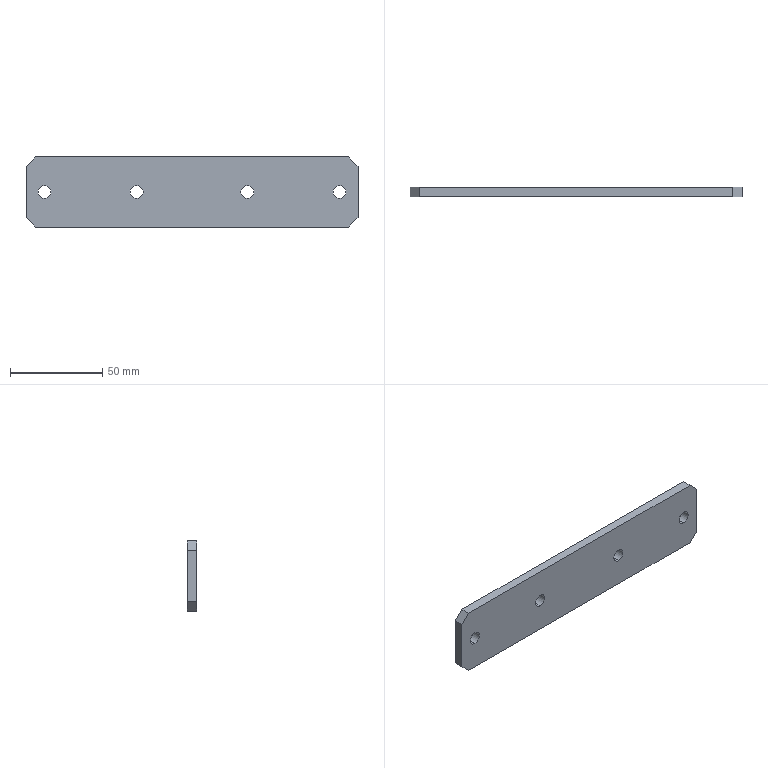Part | NX | features BREP 1 | 1 solid | 18 faces | box 180 x 5 x 38 mm | volume 33180 mm3 | plane 10 | cylinder 8 | commonest cylinder face diameters 7 x8
STEP:
#1=CARTESIAN_POINT('',(85.,5.,19.));
#2=VERTEX_POINT('',#1);
#3=CARTESIAN_POINT('',(90.,5.,14.));
#4=VERTEX_POINT('',#3);
#5=CARTESIAN_POINT('',(52.,5.,52.));
#6=DIRECTION('',(0.7071,0.,-0.7071));
#7=VECTOR('',#6,1000.);
#8=LINE('',#5,#7);
#9=EDGE_CURVE('',#2,#4,#8,.T.);
#10=ORIENTED_EDGE('',*,*,#9,.F.);
#11=CARTESIAN_POINT('',(85.,0.,19.));
#12=VERTEX_POINT('',#11);
#13=CARTESIAN_POINT('',(85.,5.,19.));
#14=DIRECTION('',(0.,1.,0.));
#15=VECTOR('',#14,1000.);
#16=LINE('',#13,#15);
#17=EDGE_CURVE('',#12,#2,#16,.T.);
#18=ORIENTED_EDGE('',*,*,#17,.F.);
#19=CARTESIAN_POINT('',(90.,0.,14.));
#20=VERTEX_POINT('',#19);
#21=CARTESIAN_POINT('',(90.,0.,14.));
#22=DIRECTION('',(-0.7071,0.,0.7071));
#23=VECTOR('',#22,1000.);
#24=LINE('',#21,#23);
#25=EDGE_CURVE('',#20,#12,#24,.T.);
#26=ORIENTED_EDGE('',*,*,#25,.F.);
#27=CARTESIAN_POINT('',(90.,5.,14.));
#28=DIRECTION('',(0.,-1.,0.));
#29=VECTOR('',#28,1000.);
#30=LINE('',#27,#29);
#31=EDGE_CURVE('',#4,#20,#30,.T.);
#32=ORIENTED_EDGE('',*,*,#31,.F.);
#33=EDGE_LOOP('',(#10,#18,#26,#32));
#34=FACE_BOUND('',#33,.T.);
#35=CARTESIAN_POINT('',(90.,5.,14.));
#36=DIRECTION('',(-0.7071,0.,-0.7071));
#37=DIRECTION('',(0.,-1.,0.));
#38=AXIS2_PLACEMENT_3D('',#35,#36,#37);
#39=PLANE('',#38);
#40=ADVANCED_FACE('',(#34),#39,.F.);
#41=CARTESIAN_POINT('',(90.,5.,-14.));
#42=VERTEX_POINT('',#41);
#43=CARTESIAN_POINT('',(85.,5.,-19.));
#44=VERTEX_POINT('',#43);
#45=CARTESIAN_POINT('',(52.,5.,-52.));
#46=DIRECTION('',(-0.7071,0.,-0.7071));
#47=VECTOR('',#46,1000.);
#48=LINE('',#45,#47);
#49=EDGE_CURVE('',#42,#44,#48,.T.);
#50=ORIENTED_EDGE('',*,*,#49,.F.);
#51=CARTESIAN_POINT('',(90.,0.,-14.));
#52=VERTEX_POINT('',#51);
#53=CARTESIAN_POINT('',(90.,5.,-14.));
#54=DIRECTION('',(0.,1.,0.));
#55=VECTOR('',#54,1000.);
#56=LINE('',#53,#55);
#57=EDGE_CURVE('',#52,#42,#56,.T.);
#58=ORIENTED_EDGE('',*,*,#57,.F.);
#59=CARTESIAN_POINT('',(85.,0.,-19.));
#60=VERTEX_POINT('',#59);
#61=CARTESIAN_POINT('',(85.,0.,-19.));
#62=DIRECTION('',(0.7071,0.,0.7071));
#63=VECTOR('',#62,1000.);
#64=LINE('',#61,#63);
#65=EDGE_CURVE('',#60,#52,#64,.T.);
#66=ORIENTED_EDGE('',*,*,#65,.F.);
#67=CARTESIAN_POINT('',(85.,5.,-19.));
#68=DIRECTION('',(0.,-1.,0.));
#69=VECTOR('',#68,1000.);
#70=LINE('',#67,#69);
#71=EDGE_CURVE('',#44,#60,#70,.T.);
#72=ORIENTED_EDGE('',*,*,#71,.F.);
#73=EDGE_LOOP('',(#50,#58,#66,#72));
#74=FACE_BOUND('',#73,.T.);
#75=CARTESIAN_POINT('',(85.,5.,-19.));
#76=DIRECTION('',(-0.7071,0.,0.7071));
#77=DIRECTION('',(0.,-1.,0.));
#78=AXIS2_PLACEMENT_3D('',#75,#76,#77);
#79=PLANE('',#78);
#80=ADVANCED_FACE('',(#74),#79,.F.);
#81=CARTESIAN_POINT('',(-90.,5.,14.));
#82=VERTEX_POINT('',#81);
#83=CARTESIAN_POINT('',(-85.,5.,19.));
#84=VERTEX_POINT('',#83);
#85=CARTESIAN_POINT('',(-52.,5.,52.));
#86=DIRECTION('',(0.7071,0.,0.7071));
#87=VECTOR('',#86,1000.);
#88=LINE('',#85,#87);
#89=EDGE_CURVE('',#82,#84,#88,.T.);
#90=ORIENTED_EDGE('',*,*,#89,.F.);
#91=CARTESIAN_POINT('',(-90.,0.,14.));
#92=VERTEX_POINT('',#91);
#93=CARTESIAN_POINT('',(-90.,5.,14.));
#94=DIRECTION('',(0.,1.,0.));
#95=VECTOR('',#94,1000.);
#96=LINE('',#93,#95);
#97=EDGE_CURVE('',#92,#82,#96,.T.);
#98=ORIENTED_EDGE('',*,*,#97,.F.);
#99=CARTESIAN_POINT('',(-85.,0.,19.));
#100=VERTEX_POINT('',#99);
#101=CARTESIAN_POINT('',(-85.,0.,19.));
#102=DIRECTION('',(-0.7071,0.,-0.7071));
#103=VECTOR('',#102,1000.);
#104=LINE('',#101,#103);
#105=EDGE_CURVE('',#100,#92,#104,.T.);
#106=ORIENTED_EDGE('',*,*,#105,.F.);
#107=CARTESIAN_POINT('',(-85.,5.,19.));
#108=DIRECTION('',(0.,-1.,0.));
#109=VECTOR('',#108,1000.);
#110=LINE('',#107,#109);
#111=EDGE_CURVE('',#84,#100,#110,.T.);
#112=ORIENTED_EDGE('',*,*,#111,.F.);
#113=EDGE_LOOP('',(#90,#98,#106,#112));
#114=FACE_BOUND('',#113,.T.);
#115=CARTESIAN_POINT('',(-85.,5.,19.));
#116=DIRECTION('',(0.7071,0.,-0.7071));
#117=DIRECTION('',(0.,-1.,0.));
#118=AXIS2_PLACEMENT_3D('',#115,#116,#117);
#119=PLANE('',#118);
#120=ADVANCED_FACE('',(#114),#119,.F.);
#121=CARTESIAN_POINT('',(-85.,5.,-19.));
#122=VERTEX_POINT('',#121);
#123=CARTESIAN_POINT('',(-90.,5.,-14.));
#124=VERTEX_POINT('',#123);
#125=CARTESIAN_POINT('',(-52.,5.,-52.));
#126=DIRECTION('',(-0.7071,0.,0.7071));
#127=VECTOR('',#126,1000.);
#128=LINE('',#125,#127);
#129=EDGE_CURVE('',#122,#124,#128,.T.);
#130=ORIENTED_EDGE('',*,*,#129,.F.);
#131=CARTESIAN_POINT('',(-85.,0.,-19.));
#132=VERTEX_POINT('',#131);
#133=CARTESIAN_POINT('',(-85.,5.,-19.));
#134=DIRECTION('',(0.,1.,0.));
#135=VECTOR('',#134,1000.);
#136=LINE('',#133,#135);
#137=EDGE_CURVE('',#132,#122,#136,.T.);
#138=ORIENTED_EDGE('',*,*,#137,.F.);
#139=CARTESIAN_POINT('',(-90.,0.,-14.));
#140=VERTEX_POINT('',#139);
#141=CARTESIAN_POINT('',(-90.,0.,-14.));
#142=DIRECTION('',(0.7071,0.,-0.7071));
#143=VECTOR('',#142,1000.);
#144=LINE('',#141,#143);
#145=EDGE_CURVE('',#140,#132,#144,.T.);
#146=ORIENTED_EDGE('',*,*,#145,.F.);
#147=CARTESIAN_POINT('',(-90.,5.,-14.));
#148=DIRECTION('',(0.,-1.,0.));
#149=VECTOR('',#148,1000.);
#150=LINE('',#147,#149);
#151=EDGE_CURVE('',#124,#140,#150,.T.);
#152=ORIENTED_EDGE('',*,*,#151,.F.);
#153=EDGE_LOOP('',(#130,#138,#146,#152));
#154=FACE_BOUND('',#153,.T.);
#155=CARTESIAN_POINT('',(-90.,5.,-14.));
#156=DIRECTION('',(0.7071,0.,0.7071));
#157=DIRECTION('',(0.,-1.,0.));
#158=AXIS2_PLACEMENT_3D('',#155,#156,#157);
#159=PLANE('',#158);
#160=ADVANCED_FACE('',(#154),#159,.F.);
#161=CARTESIAN_POINT('',(-80.,5.,-3.5));
#162=VERTEX_POINT('',#161);
#163=CARTESIAN_POINT('',(-80.,0.,-3.5));
#164=VERTEX_POINT('',#163);
#165=CARTESIAN_POINT('',(-80.,5.,-3.5));
#166=DIRECTION('',(0.,1.,0.));
#167=VECTOR('',#166,1000.);
#168=LINE('',#165,#167);
#169=EDGE_CURVE('',#162,#164,#168,.F.);
#170=ORIENTED_EDGE('',*,*,#169,.T.);
#171=CARTESIAN_POINT('',(-80.,0.,3.5));
#172=VERTEX_POINT('',#171);
#173=CARTESIAN_POINT('',(-80.,0.,0.));
#174=DIRECTION('',(0.,1.,0.));
#175=DIRECTION('',(0.,0.,1.));
#176=AXIS2_PLACEMENT_3D('',#173,#174,#175);
#177=CIRCLE('',#176,3.5);
#178=EDGE_CURVE('',#172,#164,#177,.T.);
#179=ORIENTED_EDGE('',*,*,#178,.F.);
#180=CARTESIAN_POINT('',(-80.,5.,3.5));
#181=VERTEX_POINT('',#180);
#182=CARTESIAN_POINT('',(-80.,5.,3.5));
#183=DIRECTION('',(0.,1.,0.));
#184=VECTOR('',#183,1000.);
#185=LINE('',#182,#184);
#186=EDGE_CURVE('',#181,#172,#185,.F.);
#187=ORIENTED_EDGE('',*,*,#186,.F.);
#188=CARTESIAN_POINT('',(-80.,5.,0.));
#189=DIRECTION('',(0.,1.,0.));
#190=DIRECTION('',(0.,0.,1.));
#191=AXIS2_PLACEMENT_3D('',#188,#189,#190);
#192=CIRCLE('',#191,3.5);
#193=EDGE_CURVE('',#181,#162,#192,.T.);
#194=ORIENTED_EDGE('',*,*,#193,.T.);
#195=EDGE_LOOP('',(#170,#179,#187,#194));
#196=FACE_BOUND('',#195,.T.);
#197=CARTESIAN_POINT('',(-80.,5.,0.));
#198=DIRECTION('',(0.,1.,0.));
#199=DIRECTION('',(0.,0.,1.));
#200=AXIS2_PLACEMENT_3D('',#197,#198,#199);
#201=CYLINDRICAL_SURFACE('',#200,3.5);
#202=ADVANCED_FACE('',(#196),#201,.F.);
#203=CARTESIAN_POINT('',(-30.,5.,-3.5));
#204=VERTEX_POINT('',#203);
#205=CARTESIAN_POINT('',(-30.,0.,-3.5));
#206=VERTEX_POINT('',#205);
#207=CARTESIAN_POINT('',(-30.,5.,-3.5));
#208=DIRECTION('',(0.,1.,0.));
#209=VECTOR('',#208,1000.);
#210=LINE('',#207,#209);
#211=EDGE_CURVE('',#204,#206,#210,.F.);
#212=ORIENTED_EDGE('',*,*,#211,.T.);
#213=CARTESIAN_POINT('',(-30.,0.,3.5));
#214=VERTEX_POINT('',#213);
#215=CARTESIAN_POINT('',(-30.,0.,0.));
#216=DIRECTION('',(0.,1.,0.));
#217=DIRECTION('',(0.,0.,1.));
#218=AXIS2_PLACEMENT_3D('',#215,#216,#217);
#219=CIRCLE('',#218,3.5);
#220=EDGE_CURVE('',#214,#206,#219,.T.);
#221=ORIENTED_EDGE('',*,*,#220,.F.);
#222=CARTESIAN_POINT('',(-30.,5.,3.5));
#223=VERTEX_POINT('',#222);
#224=CARTESIAN_POINT('',(-30.,5.,3.5));
#225=DIRECTION('',(0.,1.,0.));
#226=VECTOR('',#225,1000.);
#227=LINE('',#224,#226);
#228=EDGE_CURVE('',#223,#214,#227,.F.);
#229=ORIENTED_EDGE('',*,*,#228,.F.);
#230=CARTESIAN_POINT('',(-30.,5.,0.));
#231=DIRECTION('',(0.,1.,0.));
#232=DIRECTION('',(0.,0.,1.));
#233=AXIS2_PLACEMENT_3D('',#230,#231,#232);
#234=CIRCLE('',#233,3.5);
#235=EDGE_CURVE('',#223,#204,#234,.T.);
#236=ORIENTED_EDGE('',*,*,#235,.T.);
#237=EDGE_LOOP('',(#212,#221,#229,#236));
#238=FACE_BOUND('',#237,.T.);
#239=CARTESIAN_POINT('',(-30.,5.,0.));
#240=DIRECTION('',(0.,1.,0.));
#241=DIRECTION('',(0.,0.,1.));
#242=AXIS2_PLACEMENT_3D('',#239,#240,#241);
#243=CYLINDRICAL_SURFACE('',#242,3.5);
#244=ADVANCED_FACE('',(#238),#243,.F.);
#245=CARTESIAN_POINT('',(30.,5.,-3.5));
#246=VERTEX_POINT('',#245);
#247=CARTESIAN_POINT('',(30.,0.,-3.5));
#248=VERTEX_POINT('',#247);
#249=CARTESIAN_POINT('',(30.,5.,-3.5));
#250=DIRECTION('',(0.,1.,0.));
#251=VECTOR('',#250,1000.);
#252=LINE('',#249,#251);
#253=EDGE_CURVE('',#246,#248,#252,.F.);
#254=ORIENTED_EDGE('',*,*,#253,.T.);
#255=CARTESIAN_POINT('',(30.,0.,3.5));
#256=VERTEX_POINT('',#255);
#257=CARTESIAN_POINT('',(30.,0.,0.));
#258=DIRECTION('',(0.,1.,0.));
#259=DIRECTION('',(0.,0.,1.));
#260=AXIS2_PLACEMENT_3D('',#257,#258,#259);
#261=CIRCLE('',#260,3.5);
#262=EDGE_CURVE('',#256,#248,#261,.T.);
#263=ORIENTED_EDGE('',*,*,#262,.F.);
#264=CARTESIAN_POINT('',(30.,5.,3.5));
#265=VERTEX_POINT('',#264);
#266=CARTESIAN_POINT('',(30.,5.,3.5));
#267=DIRECTION('',(0.,1.,0.));
#268=VECTOR('',#267,1000.);
#269=LINE('',#266,#268);
#270=EDGE_CURVE('',#265,#256,#269,.F.);
#271=ORIENTED_EDGE('',*,*,#270,.F.);
#272=CARTESIAN_POINT('',(30.,5.,0.));
#273=DIRECTION('',(0.,1.,0.));
#274=DIRECTION('',(0.,0.,1.));
#275=AXIS2_PLACEMENT_3D('',#272,#273,#274);
#276=CIRCLE('',#275,3.5);
#277=EDGE_CURVE('',#265,#246,#276,.T.);
#278=ORIENTED_EDGE('',*,*,#277,.T.);
#279=EDGE_LOOP('',(#254,#263,#271,#278));
#280=FACE_BOUND('',#279,.T.);
#281=CARTESIAN_POINT('',(30.,5.,0.));
#282=DIRECTION('',(0.,1.,0.));
#283=DIRECTION('',(0.,0.,1.));
#284=AXIS2_PLACEMENT_3D('',#281,#282,#283);
#285=CYLINDRICAL_SURFACE('',#284,3.5);
#286=ADVANCED_FACE('',(#280),#285,.F.);
#287=CARTESIAN_POINT('',(80.,5.,-3.5));
#288=VERTEX_POINT('',#287);
#289=CARTESIAN_POINT('',(80.,0.,-3.5));
#290=VERTEX_POINT('',#289);
#291=CARTESIAN_POINT('',(80.,5.,-3.5));
#292=DIRECTION('',(0.,1.,0.));
#293=VECTOR('',#292,1000.);
#294=LINE('',#291,#293);
#295=EDGE_CURVE('',#288,#290,#294,.F.);
#296=ORIENTED_EDGE('',*,*,#295,.T.);
#297=CARTESIAN_POINT('',(80.,0.,3.5));
#298=VERTEX_POINT('',#297);
#299=CARTESIAN_POINT('',(80.,0.,0.));
#300=DIRECTION('',(0.,1.,0.));
#301=DIRECTION('',(0.,0.,1.));
#302=AXIS2_PLACEMENT_3D('',#299,#300,#301);
#303=CIRCLE('',#302,3.5);
#304=EDGE_CURVE('',#298,#290,#303,.T.);
#305=ORIENTED_EDGE('',*,*,#304,.F.);
#306=CARTESIAN_POINT('',(80.,5.,3.5));
#307=VERTEX_POINT('',#306);
#308=CARTESIAN_POINT('',(80.,5.,3.5));
#309=DIRECTION('',(0.,1.,0.));
#310=VECTOR('',#309,1000.);
#311=LINE('',#308,#310);
#312=EDGE_CURVE('',#307,#298,#311,.F.);
#313=ORIENTED_EDGE('',*,*,#312,.F.);
#314=CARTESIAN_POINT('',(80.,5.,0.));
#315=DIRECTION('',(0.,1.,0.));
#316=DIRECTION('',(0.,0.,1.));
#317=AXIS2_PLACEMENT_3D('',#314,#315,#316);
#318=CIRCLE('',#317,3.5);
#319=EDGE_CURVE('',#307,#288,#318,.T.);
#320=ORIENTED_EDGE('',*,*,#319,.T.);
#321=EDGE_LOOP('',(#296,#305,#313,#320));
#322=FACE_BOUND('',#321,.T.);
#323=CARTESIAN_POINT('',(80.,5.,0.));
#324=DIRECTION('',(0.,1.,0.));
#325=DIRECTION('',(0.,0.,1.));
#326=AXIS2_PLACEMENT_3D('',#323,#324,#325);
#327=CYLINDRICAL_SURFACE('',#326,3.5);
#328=ADVANCED_FACE('',(#322),#327,.F.);
#329=CARTESIAN_POINT('',(-90.,0.,19.));
#330=DIRECTION('',(0.,0.,1.));
#331=VECTOR('',#330,1000.);
#332=LINE('',#329,#331);
#333=EDGE_CURVE('',#140,#92,#332,.T.);
#334=ORIENTED_EDGE('',*,*,#333,.F.);
#335=ORIENTED_EDGE('',*,*,#145,.T.);
#336=CARTESIAN_POINT('',(90.,0.,-19.));
#337=DIRECTION('',(-1.,0.,0.));
#338=VECTOR('',#337,1000.);
#339=LINE('',#336,#338);
#340=EDGE_CURVE('',#60,#132,#339,.T.);
#341=ORIENTED_EDGE('',*,*,#340,.F.);
#342=ORIENTED_EDGE('',*,*,#65,.T.);
#343=CARTESIAN_POINT('',(90.,0.,19.));
#344=DIRECTION('',(0.,0.,-1.));
#345=VECTOR('',#344,1000.);
#346=LINE('',#343,#345);
#347=EDGE_CURVE('',#20,#52,#346,.T.);
#348=ORIENTED_EDGE('',*,*,#347,.F.);
#349=ORIENTED_EDGE('',*,*,#25,.T.);
#350=CARTESIAN_POINT('',(90.,0.,19.));
#351=DIRECTION('',(1.,0.,0.));
#352=VECTOR('',#351,1000.);
#353=LINE('',#350,#352);
#354=EDGE_CURVE('',#100,#12,#353,.T.);
#355=ORIENTED_EDGE('',*,*,#354,.F.);
#356=ORIENTED_EDGE('',*,*,#105,.T.);
#357=EDGE_LOOP('',(#334,#335,#341,#342,#348,#349,#355,#356));
#358=FACE_BOUND('',#357,.T.);
#359=ORIENTED_EDGE('',*,*,#304,.T.);
#360=CARTESIAN_POINT('',(80.,0.,0.));
#361=DIRECTION('',(0.,1.,0.));
#362=DIRECTION('',(0.,0.,1.));
#363=AXIS2_PLACEMENT_3D('',#360,#361,#362);
#364=CIRCLE('',#363,3.5);
#365=EDGE_CURVE('',#290,#298,#364,.T.);
#366=ORIENTED_EDGE('',*,*,#365,.T.);
#367=EDGE_LOOP('',(#359,#366));
#368=FACE_BOUND('',#367,.T.);
#369=ORIENTED_EDGE('',*,*,#262,.T.);
#370=CARTESIAN_POINT('',(30.,0.,0.));
#371=DIRECTION('',(0.,1.,0.));
#372=DIRECTION('',(0.,0.,1.));
#373=AXIS2_PLACEMENT_3D('',#370,#371,#372);
#374=CIRCLE('',#373,3.5);
#375=EDGE_CURVE('',#248,#256,#374,.T.);
#376=ORIENTED_EDGE('',*,*,#375,.T.);
#377=EDGE_LOOP('',(#369,#376));
#378=FACE_BOUND('',#377,.T.);
#379=ORIENTED_EDGE('',*,*,#220,.T.);
#380=CARTESIAN_POINT('',(-30.,0.,0.));
#381=DIRECTION('',(0.,1.,0.));
#382=DIRECTION('',(0.,0.,1.));
#383=AXIS2_PLACEMENT_3D('',#380,#381,#382);
#384=CIRCLE('',#383,3.5);
#385=EDGE_CURVE('',#206,#214,#384,.T.);
#386=ORIENTED_EDGE('',*,*,#385,.T.);
#387=EDGE_LOOP('',(#379,#386));
#388=FACE_BOUND('',#387,.T.);
#389=ORIENTED_EDGE('',*,*,#178,.T.);
#390=CARTESIAN_POINT('',(-80.,0.,0.));
#391=DIRECTION('',(0.,1.,0.));
#392=DIRECTION('',(0.,0.,1.));
#393=AXIS2_PLACEMENT_3D('',#390,#391,#392);
#394=CIRCLE('',#393,3.5);
#395=EDGE_CURVE('',#164,#172,#394,.T.);
#396=ORIENTED_EDGE('',*,*,#395,.T.);
#397=EDGE_LOOP('',(#389,#396));
#398=FACE_BOUND('',#397,.T.);
#399=CARTESIAN_POINT('',(0.,0.,0.));
#400=DIRECTION('',(0.,1.,0.));
#401=DIRECTION('',(0.,0.,1.));
#402=AXIS2_PLACEMENT_3D('',#399,#400,#401);
#403=PLANE('',#402);
#404=ADVANCED_FACE('',(#358,#368,#378,#388,#398),#403,.F.);
#405=CARTESIAN_POINT('',(90.,5.,-19.));
#406=DIRECTION('',(-1.,0.,0.));
#407=VECTOR('',#406,1000.);
#408=LINE('',#405,#407);
#409=EDGE_CURVE('',#44,#122,#408,.T.);
#410=ORIENTED_EDGE('',*,*,#409,.T.);
#411=ORIENTED_EDGE('',*,*,#129,.T.);
#412=CARTESIAN_POINT('',(-90.,5.,19.));
#413=DIRECTION('',(0.,0.,1.));
#414=VECTOR('',#413,1000.);
#415=LINE('',#412,#414);
#416=EDGE_CURVE('',#124,#82,#415,.T.);
#417=ORIENTED_EDGE('',*,*,#416,.T.);
#418=ORIENTED_EDGE('',*,*,#89,.T.);
#419=CARTESIAN_POINT('',(90.,5.,19.));
#420=DIRECTION('',(1.,0.,0.));
#421=VECTOR('',#420,1000.);
#422=LINE('',#419,#421);
#423=EDGE_CURVE('',#84,#2,#422,.T.);
#424=ORIENTED_EDGE('',*,*,#423,.T.);
#425=ORIENTED_EDGE('',*,*,#9,.T.);
#426=CARTESIAN_POINT('',(90.,5.,19.));
#427=DIRECTION('',(0.,0.,-1.));
#428=VECTOR('',#427,1000.);
#429=LINE('',#426,#428);
#430=EDGE_CURVE('',#4,#42,#429,.T.);
#431=ORIENTED_EDGE('',*,*,#430,.T.);
#432=ORIENTED_EDGE('',*,*,#49,.T.);
#433=EDGE_LOOP('',(#410,#411,#417,#418,#424,#425,#431,#432));
#434=FACE_BOUND('',#433,.T.);
#435=ORIENTED_EDGE('',*,*,#319,.F.);
#436=CARTESIAN_POINT('',(80.,5.,0.));
#437=DIRECTION('',(0.,1.,0.));
#438=DIRECTION('',(0.,0.,1.));
#439=AXIS2_PLACEMENT_3D('',#436,#437,#438);
#440=CIRCLE('',#439,3.5);
#441=EDGE_CURVE('',#288,#307,#440,.T.);
#442=ORIENTED_EDGE('',*,*,#441,.F.);
#443=EDGE_LOOP('',(#435,#442));
#444=FACE_BOUND('',#443,.T.);
#445=ORIENTED_EDGE('',*,*,#277,.F.);
#446=CARTESIAN_POINT('',(30.,5.,0.));
#447=DIRECTION('',(0.,1.,0.));
#448=DIRECTION('',(0.,0.,1.));
#449=AXIS2_PLACEMENT_3D('',#446,#447,#448);
#450=CIRCLE('',#449,3.5);
#451=EDGE_CURVE('',#246,#265,#450,.T.);
#452=ORIENTED_EDGE('',*,*,#451,.F.);
#453=EDGE_LOOP('',(#445,#452));
#454=FACE_BOUND('',#453,.T.);
#455=ORIENTED_EDGE('',*,*,#235,.F.);
#456=CARTESIAN_POINT('',(-30.,5.,0.));
#457=DIRECTION('',(0.,1.,0.));
#458=DIRECTION('',(0.,0.,1.));
#459=AXIS2_PLACEMENT_3D('',#456,#457,#458);
#460=CIRCLE('',#459,3.5);
#461=EDGE_CURVE('',#204,#223,#460,.T.);
#462=ORIENTED_EDGE('',*,*,#461,.F.);
#463=EDGE_LOOP('',(#455,#462));
#464=FACE_BOUND('',#463,.T.);
#465=ORIENTED_EDGE('',*,*,#193,.F.);
#466=CARTESIAN_POINT('',(-80.,5.,0.));
#467=DIRECTION('',(0.,1.,0.));
#468=DIRECTION('',(0.,0.,1.));
#469=AXIS2_PLACEMENT_3D('',#466,#467,#468);
#470=CIRCLE('',#469,3.5);
#471=EDGE_CURVE('',#162,#181,#470,.T.);
#472=ORIENTED_EDGE('',*,*,#471,.F.);
#473=EDGE_LOOP('',(#465,#472));
#474=FACE_BOUND('',#473,.T.);
#475=CARTESIAN_POINT('',(0.,5.,0.));
#476=DIRECTION('',(0.,1.,0.));
#477=DIRECTION('',(0.,0.,1.));
#478=AXIS2_PLACEMENT_3D('',#475,#476,#477);
#479=PLANE('',#478);
#480=ADVANCED_FACE('',(#434,#444,#454,#464,#474),#479,.T.);
#481=ORIENTED_EDGE('',*,*,#340,.T.);
#482=ORIENTED_EDGE('',*,*,#137,.T.);
#483=ORIENTED_EDGE('',*,*,#409,.F.);
#484=ORIENTED_EDGE('',*,*,#71,.T.);
#485=EDGE_LOOP('',(#481,#482,#483,#484));
#486=FACE_BOUND('',#485,.T.);
#487=CARTESIAN_POINT('',(90.,5.,-19.));
#488=DIRECTION('',(0.,0.,1.));
#489=DIRECTION('',(1.,0.,0.));
#490=AXIS2_PLACEMENT_3D('',#487,#488,#489);
#491=PLANE('',#490);
#492=ADVANCED_FACE('',(#486),#491,.F.);
#493=ORIENTED_EDGE('',*,*,#347,.T.);
#494=ORIENTED_EDGE('',*,*,#57,.T.);
#495=ORIENTED_EDGE('',*,*,#430,.F.);
#496=ORIENTED_EDGE('',*,*,#31,.T.);
#497=EDGE_LOOP('',(#493,#494,#495,#496));
#498=FACE_BOUND('',#497,.T.);
#499=CARTESIAN_POINT('',(90.,5.,19.));
#500=DIRECTION('',(-1.,0.,0.));
#501=DIRECTION('',(0.,0.,1.));
#502=AXIS2_PLACEMENT_3D('',#499,#500,#501);
#503=PLANE('',#502);
#504=ADVANCED_FACE('',(#498),#503,.F.);
#505=ORIENTED_EDGE('',*,*,#423,.F.);
#506=ORIENTED_EDGE('',*,*,#111,.T.);
#507=ORIENTED_EDGE('',*,*,#354,.T.);
#508=ORIENTED_EDGE('',*,*,#17,.T.);
#509=EDGE_LOOP('',(#505,#506,#507,#508));
#510=FACE_BOUND('',#509,.T.);
#511=CARTESIAN_POINT('',(90.,5.,19.));
#512=DIRECTION('',(0.,0.,-1.));
#513=DIRECTION('',(-1.,0.,0.));
#514=AXIS2_PLACEMENT_3D('',#511,#512,#513);
#515=PLANE('',#514);
#516=ADVANCED_FACE('',(#510),#515,.F.);
#517=ORIENTED_EDGE('',*,*,#416,.F.);
#518=ORIENTED_EDGE('',*,*,#151,.T.);
#519=ORIENTED_EDGE('',*,*,#333,.T.);
#520=ORIENTED_EDGE('',*,*,#97,.T.);
#521=EDGE_LOOP('',(#517,#518,#519,#520));
#522=FACE_BOUND('',#521,.T.);
#523=CARTESIAN_POINT('',(-90.,5.,19.));
#524=DIRECTION('',(1.,0.,0.));
#525=DIRECTION('',(0.,0.,-1.));
#526=AXIS2_PLACEMENT_3D('',#523,#524,#525);
#527=PLANE('',#526);
#528=ADVANCED_FACE('',(#522),#527,.F.);
#529=ORIENTED_EDGE('',*,*,#365,.F.);
#530=ORIENTED_EDGE('',*,*,#295,.F.);
#531=ORIENTED_EDGE('',*,*,#441,.T.);
#532=ORIENTED_EDGE('',*,*,#312,.T.);
#533=EDGE_LOOP('',(#529,#530,#531,#532));
#534=FACE_BOUND('',#533,.T.);
#535=CARTESIAN_POINT('',(80.,5.,0.));
#536=DIRECTION('',(0.,1.,0.));
#537=DIRECTION('',(0.,0.,1.));
#538=AXIS2_PLACEMENT_3D('',#535,#536,#537);
#539=CYLINDRICAL_SURFACE('',#538,3.5);
#540=ADVANCED_FACE('',(#534),#539,.F.);
#541=ORIENTED_EDGE('',*,*,#375,.F.);
#542=ORIENTED_EDGE('',*,*,#253,.F.);
#543=ORIENTED_EDGE('',*,*,#451,.T.);
#544=ORIENTED_EDGE('',*,*,#270,.T.);
#545=EDGE_LOOP('',(#541,#542,#543,#544));
#546=FACE_BOUND('',#545,.T.);
#547=CARTESIAN_POINT('',(30.,5.,0.));
#548=DIRECTION('',(0.,1.,0.));
#549=DIRECTION('',(0.,0.,1.));
#550=AXIS2_PLACEMENT_3D('',#547,#548,#549);
#551=CYLINDRICAL_SURFACE('',#550,3.5);
#552=ADVANCED_FACE('',(#546),#551,.F.);
#553=ORIENTED_EDGE('',*,*,#385,.F.);
#554=ORIENTED_EDGE('',*,*,#211,.F.);
#555=ORIENTED_EDGE('',*,*,#461,.T.);
#556=ORIENTED_EDGE('',*,*,#228,.T.);
#557=EDGE_LOOP('',(#553,#554,#555,#556));
#558=FACE_BOUND('',#557,.T.);
#559=CARTESIAN_POINT('',(-30.,5.,0.));
#560=DIRECTION('',(0.,1.,0.));
#561=DIRECTION('',(0.,0.,1.));
#562=AXIS2_PLACEMENT_3D('',#559,#560,#561);
#563=CYLINDRICAL_SURFACE('',#562,3.5);
#564=ADVANCED_FACE('',(#558),#563,.F.);
#565=ORIENTED_EDGE('',*,*,#395,.F.);
#566=ORIENTED_EDGE('',*,*,#169,.F.);
#567=ORIENTED_EDGE('',*,*,#471,.T.);
#568=ORIENTED_EDGE('',*,*,#186,.T.);
#569=EDGE_LOOP('',(#565,#566,#567,#568));
#570=FACE_BOUND('',#569,.T.);
#571=CARTESIAN_POINT('',(-80.,5.,0.));
#572=DIRECTION('',(0.,1.,0.));
#573=DIRECTION('',(0.,0.,1.));
#574=AXIS2_PLACEMENT_3D('',#571,#572,#573);
#575=CYLINDRICAL_SURFACE('',#574,3.5);
#576=ADVANCED_FACE('',(#570),#575,.F.);
#577=CLOSED_SHELL('',(#40,#80,#120,#160,#202,#244,#286,#328,#404,#480,#492,#504,#516,#528,#540,#552,#564,#576));
#578=MANIFOLD_SOLID_BREP('',#577);
#579=(LENGTH_UNIT()NAMED_UNIT(*)SI_UNIT(.MILLI.,.METRE.));
#580=UNCERTAINTY_MEASURE_WITH_UNIT(LENGTH_MEASURE(0.00001),#579,'','');
#581=(NAMED_UNIT(*)PLANE_ANGLE_UNIT()SI_UNIT($,.RADIAN.));
#582=(NAMED_UNIT(*)SI_UNIT($,.STERADIAN.)SOLID_ANGLE_UNIT());
#583=(GEOMETRIC_REPRESENTATION_CONTEXT(3)GLOBAL_UNCERTAINTY_ASSIGNED_CONTEXT((#580))GLOBAL_UNIT_ASSIGNED_CONTEXT((#579,#581,#582))REPRESENTATION_CONTEXT('',''));
#584=ADVANCED_BREP_SHAPE_REPRESENTATION('',(#578),#583);